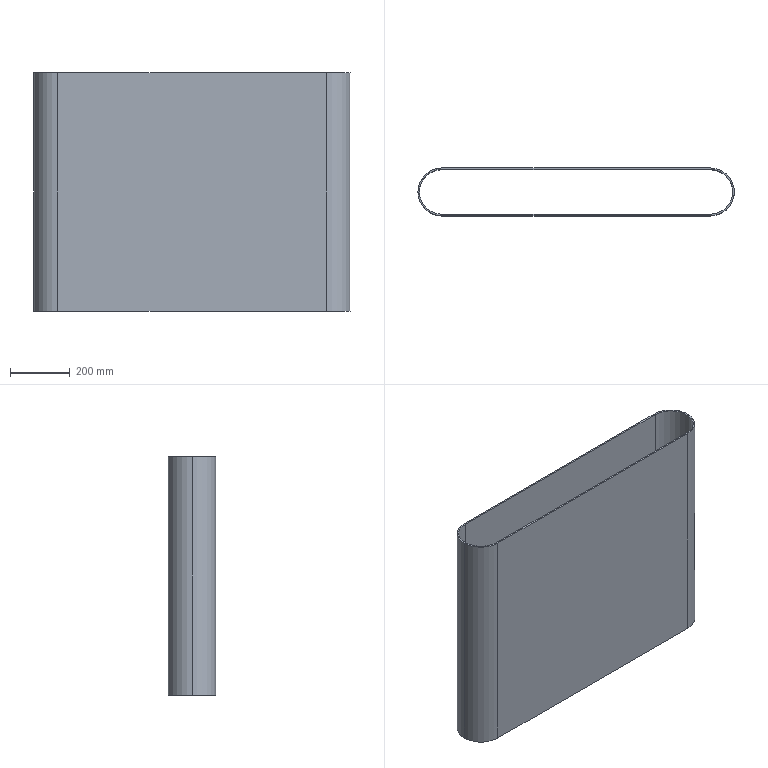Part | SolidWorks | features ExtruThin 1 | 1 solid | 12 faces | box 1060 x 160 x 800 mm | volume 9147787 mm3 | cylinder 6 | plane 6 | commonest cylinder face diameters 150 x3 160 x3
STEP:
#1=CARTESIAN_POINT('',(-450.,80.061,800.));
#2=VERTEX_POINT('',#1);
#3=CARTESIAN_POINT('',(-525.,5.061,800.));
#4=VERTEX_POINT('',#3);
#5=CARTESIAN_POINT('',(-450.,5.061,800.));
#6=DIRECTION('',(0.,0.,1.));
#7=DIRECTION('',(1.,0.,0.));
#8=AXIS2_PLACEMENT_3D('',#5,#6,#7);
#9=CIRCLE('',#8,75.);
#10=EDGE_CURVE('',#2,#4,#9,.T.);
#11=ORIENTED_EDGE('',*,*,#10,.T.);
#12=CARTESIAN_POINT('',(-525.,5.061,0.));
#13=VERTEX_POINT('',#12);
#14=CARTESIAN_POINT('',(-525.,5.061,800.));
#15=DIRECTION('',(0.,0.,-1.));
#16=VECTOR('',#15,1000.);
#17=LINE('',#14,#16);
#18=EDGE_CURVE('',#4,#13,#17,.T.);
#19=ORIENTED_EDGE('',*,*,#18,.T.);
#20=CARTESIAN_POINT('',(-450.,80.061,0.));
#21=VERTEX_POINT('',#20);
#22=CARTESIAN_POINT('',(-450.,5.061,0.));
#23=DIRECTION('',(0.,0.,1.));
#24=DIRECTION('',(1.,0.,0.));
#25=AXIS2_PLACEMENT_3D('',#22,#23,#24);
#26=CIRCLE('',#25,75.);
#27=EDGE_CURVE('',#21,#13,#26,.T.);
#28=ORIENTED_EDGE('',*,*,#27,.F.);
#29=CARTESIAN_POINT('',(-450.,80.061,800.));
#30=DIRECTION('',(0.,0.,-1.));
#31=VECTOR('',#30,1000.);
#32=LINE('',#29,#31);
#33=EDGE_CURVE('',#2,#21,#32,.T.);
#34=ORIENTED_EDGE('',*,*,#33,.F.);
#35=EDGE_LOOP('',(#11,#19,#28,#34));
#36=FACE_OUTER_BOUND('',#35,.T.);
#37=CARTESIAN_POINT('',(-450.,5.061,800.));
#38=DIRECTION('',(0.,0.,-1.));
#39=DIRECTION('',(-1.,0.,0.));
#40=AXIS2_PLACEMENT_3D('',#37,#38,#39);
#41=CYLINDRICAL_SURFACE('',#40,75.);
#42=ADVANCED_FACE('',(#36),#41,.F.);
#43=CARTESIAN_POINT('',(-530.,5.061,800.));
#44=VERTEX_POINT('',#43);
#45=CARTESIAN_POINT('',(-450.,-74.939,800.));
#46=VERTEX_POINT('',#45);
#47=CARTESIAN_POINT('',(-450.,5.061,800.));
#48=DIRECTION('',(0.,0.,1.));
#49=DIRECTION('',(1.,0.,0.));
#50=AXIS2_PLACEMENT_3D('',#47,#48,#49);
#51=CIRCLE('',#50,80.);
#52=EDGE_CURVE('',#44,#46,#51,.T.);
#53=ORIENTED_EDGE('',*,*,#52,.F.);
#54=CARTESIAN_POINT('',(-530.,5.061,0.));
#55=VERTEX_POINT('',#54);
#56=CARTESIAN_POINT('',(-530.,5.061,800.));
#57=DIRECTION('',(0.,0.,-1.));
#58=VECTOR('',#57,1000.);
#59=LINE('',#56,#58);
#60=EDGE_CURVE('',#44,#55,#59,.T.);
#61=ORIENTED_EDGE('',*,*,#60,.T.);
#62=CARTESIAN_POINT('',(-450.,-74.939,0.));
#63=VERTEX_POINT('',#62);
#64=CARTESIAN_POINT('',(-450.,5.061,0.));
#65=DIRECTION('',(0.,0.,1.));
#66=DIRECTION('',(1.,0.,0.));
#67=AXIS2_PLACEMENT_3D('',#64,#65,#66);
#68=CIRCLE('',#67,80.);
#69=EDGE_CURVE('',#55,#63,#68,.T.);
#70=ORIENTED_EDGE('',*,*,#69,.T.);
#71=CARTESIAN_POINT('',(-450.,-74.939,800.));
#72=DIRECTION('',(0.,0.,-1.));
#73=VECTOR('',#72,1000.);
#74=LINE('',#71,#73);
#75=EDGE_CURVE('',#46,#63,#74,.T.);
#76=ORIENTED_EDGE('',*,*,#75,.F.);
#77=EDGE_LOOP('',(#53,#61,#70,#76));
#78=FACE_OUTER_BOUND('',#77,.T.);
#79=CARTESIAN_POINT('',(-450.,5.061,800.));
#80=DIRECTION('',(0.,0.,-1.));
#81=DIRECTION('',(-1.,0.,0.));
#82=AXIS2_PLACEMENT_3D('',#79,#80,#81);
#83=CYLINDRICAL_SURFACE('',#82,80.);
#84=ADVANCED_FACE('',(#78),#83,.T.);
#85=CARTESIAN_POINT('',(450.,-74.939,800.));
#86=VERTEX_POINT('',#85);
#87=CARTESIAN_POINT('',(-450.,-74.939,800.));
#88=DIRECTION('',(1.,0.,0.));
#89=VECTOR('',#88,1000.);
#90=LINE('',#87,#89);
#91=EDGE_CURVE('',#46,#86,#90,.T.);
#92=ORIENTED_EDGE('',*,*,#91,.T.);
#93=CARTESIAN_POINT('',(450.,85.061,800.));
#94=VERTEX_POINT('',#93);
#95=CARTESIAN_POINT('',(450.,5.061,800.));
#96=DIRECTION('',(0.,0.,1.));
#97=DIRECTION('',(1.,0.,0.));
#98=AXIS2_PLACEMENT_3D('',#95,#96,#97);
#99=CIRCLE('',#98,80.);
#100=EDGE_CURVE('',#86,#94,#99,.T.);
#101=ORIENTED_EDGE('',*,*,#100,.T.);
#102=CARTESIAN_POINT('',(-450.,85.061,800.));
#103=VERTEX_POINT('',#102);
#104=CARTESIAN_POINT('',(-450.,85.061,800.));
#105=DIRECTION('',(1.,0.,0.));
#106=VECTOR('',#105,1000.);
#107=LINE('',#104,#106);
#108=EDGE_CURVE('',#103,#94,#107,.T.);
#109=ORIENTED_EDGE('',*,*,#108,.F.);
#110=CARTESIAN_POINT('',(-450.,5.061,800.));
#111=DIRECTION('',(0.,0.,1.));
#112=DIRECTION('',(1.,0.,0.));
#113=AXIS2_PLACEMENT_3D('',#110,#111,#112);
#114=CIRCLE('',#113,80.);
#115=EDGE_CURVE('',#103,#44,#114,.T.);
#116=ORIENTED_EDGE('',*,*,#115,.T.);
#117=ORIENTED_EDGE('',*,*,#52,.T.);
#118=EDGE_LOOP('',(#92,#101,#109,#116,#117));
#119=FACE_OUTER_BOUND('',#118,.T.);
#120=CARTESIAN_POINT('',(450.,-69.939,800.));
#121=VERTEX_POINT('',#120);
#122=CARTESIAN_POINT('',(450.,80.061,800.));
#123=VERTEX_POINT('',#122);
#124=CARTESIAN_POINT('',(450.,5.061,800.));
#125=DIRECTION('',(0.,0.,1.));
#126=DIRECTION('',(1.,0.,0.));
#127=AXIS2_PLACEMENT_3D('',#124,#125,#126);
#128=CIRCLE('',#127,75.);
#129=EDGE_CURVE('',#121,#123,#128,.T.);
#130=ORIENTED_EDGE('',*,*,#129,.F.);
#131=CARTESIAN_POINT('',(-450.,-69.939,800.));
#132=VERTEX_POINT('',#131);
#133=CARTESIAN_POINT('',(-450.,-69.939,800.));
#134=DIRECTION('',(1.,0.,0.));
#135=VECTOR('',#134,1000.);
#136=LINE('',#133,#135);
#137=EDGE_CURVE('',#132,#121,#136,.T.);
#138=ORIENTED_EDGE('',*,*,#137,.F.);
#139=CARTESIAN_POINT('',(-450.,5.061,800.));
#140=DIRECTION('',(0.,0.,1.));
#141=DIRECTION('',(1.,0.,0.));
#142=AXIS2_PLACEMENT_3D('',#139,#140,#141);
#143=CIRCLE('',#142,75.);
#144=EDGE_CURVE('',#4,#132,#143,.T.);
#145=ORIENTED_EDGE('',*,*,#144,.F.);
#146=ORIENTED_EDGE('',*,*,#10,.F.);
#147=CARTESIAN_POINT('',(-450.,80.061,800.));
#148=DIRECTION('',(1.,0.,0.));
#149=VECTOR('',#148,1000.);
#150=LINE('',#147,#149);
#151=EDGE_CURVE('',#2,#123,#150,.T.);
#152=ORIENTED_EDGE('',*,*,#151,.T.);
#153=EDGE_LOOP('',(#130,#138,#145,#146,#152));
#154=FACE_BOUND('',#153,.T.);
#155=CARTESIAN_POINT('',(450.,5.061,800.));
#156=DIRECTION('',(0.,0.,1.));
#157=DIRECTION('',(1.,0.,0.));
#158=AXIS2_PLACEMENT_3D('',#155,#156,#157);
#159=PLANE('',#158);
#160=ADVANCED_FACE('',(#119,#154),#159,.T.);
#161=CARTESIAN_POINT('',(450.,-74.939,0.));
#162=VERTEX_POINT('',#161);
#163=CARTESIAN_POINT('',(-450.,-74.939,0.));
#164=DIRECTION('',(1.,0.,0.));
#165=VECTOR('',#164,1000.);
#166=LINE('',#163,#165);
#167=EDGE_CURVE('',#63,#162,#166,.T.);
#168=ORIENTED_EDGE('',*,*,#167,.F.);
#169=ORIENTED_EDGE('',*,*,#69,.F.);
#170=CARTESIAN_POINT('',(-450.,85.061,0.));
#171=VERTEX_POINT('',#170);
#172=CARTESIAN_POINT('',(-450.,5.061,0.));
#173=DIRECTION('',(0.,0.,1.));
#174=DIRECTION('',(1.,0.,0.));
#175=AXIS2_PLACEMENT_3D('',#172,#173,#174);
#176=CIRCLE('',#175,80.);
#177=EDGE_CURVE('',#171,#55,#176,.T.);
#178=ORIENTED_EDGE('',*,*,#177,.F.);
#179=CARTESIAN_POINT('',(450.,85.061,0.));
#180=VERTEX_POINT('',#179);
#181=CARTESIAN_POINT('',(-450.,85.061,0.));
#182=DIRECTION('',(1.,0.,0.));
#183=VECTOR('',#182,1000.);
#184=LINE('',#181,#183);
#185=EDGE_CURVE('',#171,#180,#184,.T.);
#186=ORIENTED_EDGE('',*,*,#185,.T.);
#187=CARTESIAN_POINT('',(450.,5.061,0.));
#188=DIRECTION('',(0.,0.,1.));
#189=DIRECTION('',(1.,0.,0.));
#190=AXIS2_PLACEMENT_3D('',#187,#188,#189);
#191=CIRCLE('',#190,80.);
#192=EDGE_CURVE('',#162,#180,#191,.T.);
#193=ORIENTED_EDGE('',*,*,#192,.F.);
#194=EDGE_LOOP('',(#168,#169,#178,#186,#193));
#195=FACE_OUTER_BOUND('',#194,.T.);
#196=CARTESIAN_POINT('',(-450.,-69.939,0.));
#197=VERTEX_POINT('',#196);
#198=CARTESIAN_POINT('',(450.,-69.939,0.));
#199=VERTEX_POINT('',#198);
#200=CARTESIAN_POINT('',(-450.,-69.939,0.));
#201=DIRECTION('',(1.,0.,0.));
#202=VECTOR('',#201,1000.);
#203=LINE('',#200,#202);
#204=EDGE_CURVE('',#197,#199,#203,.T.);
#205=ORIENTED_EDGE('',*,*,#204,.T.);
#206=CARTESIAN_POINT('',(450.,80.061,0.));
#207=VERTEX_POINT('',#206);
#208=CARTESIAN_POINT('',(450.,5.061,0.));
#209=DIRECTION('',(0.,0.,1.));
#210=DIRECTION('',(1.,0.,0.));
#211=AXIS2_PLACEMENT_3D('',#208,#209,#210);
#212=CIRCLE('',#211,75.);
#213=EDGE_CURVE('',#199,#207,#212,.T.);
#214=ORIENTED_EDGE('',*,*,#213,.T.);
#215=CARTESIAN_POINT('',(-450.,80.061,0.));
#216=DIRECTION('',(1.,0.,0.));
#217=VECTOR('',#216,1000.);
#218=LINE('',#215,#217);
#219=EDGE_CURVE('',#21,#207,#218,.T.);
#220=ORIENTED_EDGE('',*,*,#219,.F.);
#221=ORIENTED_EDGE('',*,*,#27,.T.);
#222=CARTESIAN_POINT('',(-450.,5.061,0.));
#223=DIRECTION('',(0.,0.,1.));
#224=DIRECTION('',(1.,0.,0.));
#225=AXIS2_PLACEMENT_3D('',#222,#223,#224);
#226=CIRCLE('',#225,75.);
#227=EDGE_CURVE('',#13,#197,#226,.T.);
#228=ORIENTED_EDGE('',*,*,#227,.T.);
#229=EDGE_LOOP('',(#205,#214,#220,#221,#228));
#230=FACE_BOUND('',#229,.T.);
#231=CARTESIAN_POINT('',(450.,5.061,0.));
#232=DIRECTION('',(0.,0.,1.));
#233=DIRECTION('',(1.,0.,0.));
#234=AXIS2_PLACEMENT_3D('',#231,#232,#233);
#235=PLANE('',#234);
#236=ADVANCED_FACE('',(#195,#230),#235,.F.);
#237=ORIENTED_EDGE('',*,*,#167,.T.);
#238=CARTESIAN_POINT('',(450.,-74.939,800.));
#239=DIRECTION('',(0.,0.,-1.));
#240=VECTOR('',#239,1000.);
#241=LINE('',#238,#240);
#242=EDGE_CURVE('',#86,#162,#241,.T.);
#243=ORIENTED_EDGE('',*,*,#242,.F.);
#244=ORIENTED_EDGE('',*,*,#91,.F.);
#245=ORIENTED_EDGE('',*,*,#75,.T.);
#246=EDGE_LOOP('',(#237,#243,#244,#245));
#247=FACE_OUTER_BOUND('',#246,.T.);
#248=CARTESIAN_POINT('',(-450.,-74.939,800.));
#249=DIRECTION('',(0.,1.,0.));
#250=DIRECTION('',(0.,0.,1.));
#251=AXIS2_PLACEMENT_3D('',#248,#249,#250);
#252=PLANE('',#251);
#253=ADVANCED_FACE('',(#247),#252,.F.);
#254=ORIENTED_EDGE('',*,*,#192,.T.);
#255=CARTESIAN_POINT('',(450.,85.061,800.));
#256=DIRECTION('',(0.,0.,-1.));
#257=VECTOR('',#256,1000.);
#258=LINE('',#255,#257);
#259=EDGE_CURVE('',#94,#180,#258,.T.);
#260=ORIENTED_EDGE('',*,*,#259,.F.);
#261=ORIENTED_EDGE('',*,*,#100,.F.);
#262=ORIENTED_EDGE('',*,*,#242,.T.);
#263=EDGE_LOOP('',(#254,#260,#261,#262));
#264=FACE_OUTER_BOUND('',#263,.T.);
#265=CARTESIAN_POINT('',(450.,5.061,800.));
#266=DIRECTION('',(0.,0.,-1.));
#267=DIRECTION('',(-1.,0.,0.));
#268=AXIS2_PLACEMENT_3D('',#265,#266,#267);
#269=CYLINDRICAL_SURFACE('',#268,80.);
#270=ADVANCED_FACE('',(#264),#269,.T.);
#271=ORIENTED_EDGE('',*,*,#185,.F.);
#272=CARTESIAN_POINT('',(-450.,85.061,800.));
#273=DIRECTION('',(0.,0.,-1.));
#274=VECTOR('',#273,1000.);
#275=LINE('',#272,#274);
#276=EDGE_CURVE('',#103,#171,#275,.T.);
#277=ORIENTED_EDGE('',*,*,#276,.F.);
#278=ORIENTED_EDGE('',*,*,#108,.T.);
#279=ORIENTED_EDGE('',*,*,#259,.T.);
#280=EDGE_LOOP('',(#271,#277,#278,#279));
#281=FACE_OUTER_BOUND('',#280,.T.);
#282=CARTESIAN_POINT('',(-450.,85.061,800.));
#283=DIRECTION('',(0.,1.,0.));
#284=DIRECTION('',(-1.,0.,0.));
#285=AXIS2_PLACEMENT_3D('',#282,#283,#284);
#286=PLANE('',#285);
#287=ADVANCED_FACE('',(#281),#286,.T.);
#288=ORIENTED_EDGE('',*,*,#60,.F.);
#289=ORIENTED_EDGE('',*,*,#115,.F.);
#290=ORIENTED_EDGE('',*,*,#276,.T.);
#291=ORIENTED_EDGE('',*,*,#177,.T.);
#292=EDGE_LOOP('',(#288,#289,#290,#291));
#293=FACE_OUTER_BOUND('',#292,.T.);
#294=CARTESIAN_POINT('',(-450.,5.061,800.));
#295=DIRECTION('',(0.,0.,-1.));
#296=DIRECTION('',(-1.,0.,0.));
#297=AXIS2_PLACEMENT_3D('',#294,#295,#296);
#298=CYLINDRICAL_SURFACE('',#297,80.);
#299=ADVANCED_FACE('',(#293),#298,.T.);
#300=ORIENTED_EDGE('',*,*,#204,.F.);
#301=CARTESIAN_POINT('',(-450.,-69.939,800.));
#302=DIRECTION('',(0.,0.,-1.));
#303=VECTOR('',#302,1000.);
#304=LINE('',#301,#303);
#305=EDGE_CURVE('',#132,#197,#304,.T.);
#306=ORIENTED_EDGE('',*,*,#305,.F.);
#307=ORIENTED_EDGE('',*,*,#137,.T.);
#308=CARTESIAN_POINT('',(450.,-69.939,800.));
#309=DIRECTION('',(0.,0.,-1.));
#310=VECTOR('',#309,1000.);
#311=LINE('',#308,#310);
#312=EDGE_CURVE('',#121,#199,#311,.T.);
#313=ORIENTED_EDGE('',*,*,#312,.T.);
#314=EDGE_LOOP('',(#300,#306,#307,#313));
#315=FACE_OUTER_BOUND('',#314,.T.);
#316=CARTESIAN_POINT('',(-450.,-69.939,800.));
#317=DIRECTION('',(0.,1.,0.));
#318=DIRECTION('',(0.,0.,1.));
#319=AXIS2_PLACEMENT_3D('',#316,#317,#318);
#320=PLANE('',#319);
#321=ADVANCED_FACE('',(#315),#320,.T.);
#322=ORIENTED_EDGE('',*,*,#213,.F.);
#323=ORIENTED_EDGE('',*,*,#312,.F.);
#324=ORIENTED_EDGE('',*,*,#129,.T.);
#325=CARTESIAN_POINT('',(450.,80.061,800.));
#326=DIRECTION('',(0.,0.,-1.));
#327=VECTOR('',#326,1000.);
#328=LINE('',#325,#327);
#329=EDGE_CURVE('',#123,#207,#328,.T.);
#330=ORIENTED_EDGE('',*,*,#329,.T.);
#331=EDGE_LOOP('',(#322,#323,#324,#330));
#332=FACE_OUTER_BOUND('',#331,.T.);
#333=CARTESIAN_POINT('',(450.,5.061,800.));
#334=DIRECTION('',(0.,0.,-1.));
#335=DIRECTION('',(-1.,0.,0.));
#336=AXIS2_PLACEMENT_3D('',#333,#334,#335);
#337=CYLINDRICAL_SURFACE('',#336,75.);
#338=ADVANCED_FACE('',(#332),#337,.F.);
#339=ORIENTED_EDGE('',*,*,#219,.T.);
#340=ORIENTED_EDGE('',*,*,#329,.F.);
#341=ORIENTED_EDGE('',*,*,#151,.F.);
#342=ORIENTED_EDGE('',*,*,#33,.T.);
#343=EDGE_LOOP('',(#339,#340,#341,#342));
#344=FACE_OUTER_BOUND('',#343,.T.);
#345=CARTESIAN_POINT('',(-450.,80.061,800.));
#346=DIRECTION('',(0.,1.,0.));
#347=DIRECTION('',(-1.,0.,0.));
#348=AXIS2_PLACEMENT_3D('',#345,#346,#347);
#349=PLANE('',#348);
#350=ADVANCED_FACE('',(#344),#349,.F.);
#351=ORIENTED_EDGE('',*,*,#18,.F.);
#352=ORIENTED_EDGE('',*,*,#144,.T.);
#353=ORIENTED_EDGE('',*,*,#305,.T.);
#354=ORIENTED_EDGE('',*,*,#227,.F.);
#355=EDGE_LOOP('',(#351,#352,#353,#354));
#356=FACE_OUTER_BOUND('',#355,.T.);
#357=CARTESIAN_POINT('',(-450.,5.061,800.));
#358=DIRECTION('',(0.,0.,-1.));
#359=DIRECTION('',(-1.,0.,0.));
#360=AXIS2_PLACEMENT_3D('',#357,#358,#359);
#361=CYLINDRICAL_SURFACE('',#360,75.);
#362=ADVANCED_FACE('',(#356),#361,.F.);
#363=CLOSED_SHELL('',(#42,#84,#160,#236,#253,#270,#287,#299,#321,#338,#350,#362));
#364=MANIFOLD_SOLID_BREP('',#363);
#365=CARTESIAN_POINT('',(0.,0.,0.));
#366=DIRECTION('',(0.,0.,1.));
#367=DIRECTION('',(1.,0.,0.));
#368=AXIS2_PLACEMENT_3D('',#365,#366,#367);
#369=(LENGTH_UNIT()NAMED_UNIT(*)SI_UNIT(.MILLI.,.METRE.));
#370=UNCERTAINTY_MEASURE_WITH_UNIT(LENGTH_MEASURE(0.00001),#369,'','');
#371=(NAMED_UNIT(*)PLANE_ANGLE_UNIT()SI_UNIT($,.RADIAN.));
#372=(NAMED_UNIT(*)SI_UNIT($,.STERADIAN.)SOLID_ANGLE_UNIT());
#373=(GEOMETRIC_REPRESENTATION_CONTEXT(3)GLOBAL_UNCERTAINTY_ASSIGNED_CONTEXT((#370))GLOBAL_UNIT_ASSIGNED_CONTEXT((#369,#371,#372))REPRESENTATION_CONTEXT('',''));
#374=ADVANCED_BREP_SHAPE_REPRESENTATION('',(#364,#368),#373);